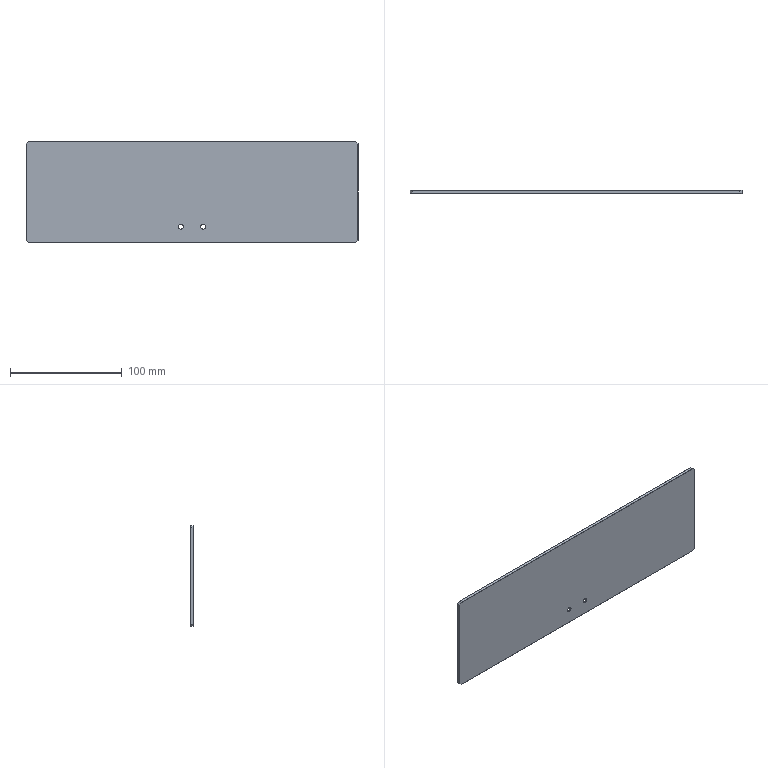Part | SolidWorks | features Chamfer 3, Extrusion 1, HoleWzd 1 | 1 solid | 34 faces | box 297 x 3 x 90 mm | volume 79946 mm3 | plane 26 | cone 4 | cylinder 4 | commonest cylinder face diameters 4.5 x4
STEP:
#1=CARTESIAN_POINT('',(-10.,0.77,-33.25));
#2=VERTEX_POINT('',#1);
#3=CARTESIAN_POINT('',(-10.,0.77,-28.75));
#4=VERTEX_POINT('',#3);
#5=CARTESIAN_POINT('',(-10.,0.77,-31.));
#6=DIRECTION('',(0.,1.,0.));
#7=DIRECTION('',(0.,0.,1.));
#8=AXIS2_PLACEMENT_3D('',#5,#6,#7);
#9=CIRCLE('',#8,2.25);
#10=EDGE_CURVE('',#2,#4,#9,.T.);
#11=ORIENTED_EDGE('',*,*,#10,.F.);
#12=CARTESIAN_POINT('',(-10.,3.,-35.48));
#13=VERTEX_POINT('',#12);
#14=CARTESIAN_POINT('',(-10.,3.,-35.48));
#15=DIRECTION('',(0.,0.7071,-0.7071));
#16=VECTOR('',#15,1000.);
#17=LINE('',#14,#16);
#18=EDGE_CURVE('',#2,#13,#17,.T.);
#19=ORIENTED_EDGE('',*,*,#18,.T.);
#20=CARTESIAN_POINT('',(-10.,3.,-26.52));
#21=VERTEX_POINT('',#20);
#22=CARTESIAN_POINT('',(-10.,3.,-31.));
#23=DIRECTION('',(0.,1.,0.));
#24=DIRECTION('',(0.,0.,1.));
#25=AXIS2_PLACEMENT_3D('',#22,#23,#24);
#26=CIRCLE('',#25,4.48);
#27=EDGE_CURVE('',#13,#21,#26,.T.);
#28=ORIENTED_EDGE('',*,*,#27,.T.);
#29=CARTESIAN_POINT('',(-10.,3.,-26.52));
#30=DIRECTION('',(0.,0.7071,0.7071));
#31=VECTOR('',#30,1000.);
#32=LINE('',#29,#31);
#33=EDGE_CURVE('',#4,#21,#32,.T.);
#34=ORIENTED_EDGE('',*,*,#33,.F.);
#35=EDGE_LOOP('',(#11,#19,#28,#34));
#36=FACE_OUTER_BOUND('',#35,.T.);
#37=CARTESIAN_POINT('',(-10.,3.,-31.));
#38=DIRECTION('',(0.,1.,0.));
#39=DIRECTION('',(0.,0.,1.));
#40=AXIS2_PLACEMENT_3D('',#37,#38,#39);
#41=CONICAL_SURFACE('',#40,4.48,0.7854);
#42=ADVANCED_FACE('',(#36),#41,.F.);
#43=CARTESIAN_POINT('',(-10.,0.,-33.25));
#44=VERTEX_POINT('',#43);
#45=CARTESIAN_POINT('',(-10.,0.,-28.75));
#46=VERTEX_POINT('',#45);
#47=CARTESIAN_POINT('',(-10.,0.,-31.));
#48=DIRECTION('',(0.,1.,0.));
#49=DIRECTION('',(0.,0.,1.));
#50=AXIS2_PLACEMENT_3D('',#47,#48,#49);
#51=CIRCLE('',#50,2.25);
#52=EDGE_CURVE('',#44,#46,#51,.T.);
#53=ORIENTED_EDGE('',*,*,#52,.F.);
#54=CARTESIAN_POINT('',(-10.,3.,-33.25));
#55=DIRECTION('',(0.,1.,0.));
#56=VECTOR('',#55,1000.);
#57=LINE('',#54,#56);
#58=EDGE_CURVE('',#44,#2,#57,.T.);
#59=ORIENTED_EDGE('',*,*,#58,.T.);
#60=ORIENTED_EDGE('',*,*,#10,.T.);
#61=CARTESIAN_POINT('',(-10.,3.,-28.75));
#62=DIRECTION('',(0.,1.,0.));
#63=VECTOR('',#62,1000.);
#64=LINE('',#61,#63);
#65=EDGE_CURVE('',#46,#4,#64,.T.);
#66=ORIENTED_EDGE('',*,*,#65,.F.);
#67=EDGE_LOOP('',(#53,#59,#60,#66));
#68=FACE_OUTER_BOUND('',#67,.T.);
#69=CARTESIAN_POINT('',(-10.,3.,-31.));
#70=DIRECTION('',(0.,1.,0.));
#71=DIRECTION('',(0.,0.,1.));
#72=AXIS2_PLACEMENT_3D('',#69,#70,#71);
#73=CYLINDRICAL_SURFACE('',#72,2.25);
#74=ADVANCED_FACE('',(#68),#73,.F.);
#75=CARTESIAN_POINT('',(10.,0.77,-33.25));
#76=VERTEX_POINT('',#75);
#77=CARTESIAN_POINT('',(10.,0.77,-28.75));
#78=VERTEX_POINT('',#77);
#79=CARTESIAN_POINT('',(10.,0.77,-31.));
#80=DIRECTION('',(0.,1.,0.));
#81=DIRECTION('',(0.,0.,1.));
#82=AXIS2_PLACEMENT_3D('',#79,#80,#81);
#83=CIRCLE('',#82,2.25);
#84=EDGE_CURVE('',#76,#78,#83,.T.);
#85=ORIENTED_EDGE('',*,*,#84,.F.);
#86=CARTESIAN_POINT('',(10.,3.,-35.48));
#87=VERTEX_POINT('',#86);
#88=CARTESIAN_POINT('',(10.,3.,-35.48));
#89=DIRECTION('',(0.,0.7071,-0.7071));
#90=VECTOR('',#89,1000.);
#91=LINE('',#88,#90);
#92=EDGE_CURVE('',#76,#87,#91,.T.);
#93=ORIENTED_EDGE('',*,*,#92,.T.);
#94=CARTESIAN_POINT('',(10.,3.,-26.52));
#95=VERTEX_POINT('',#94);
#96=CARTESIAN_POINT('',(10.,3.,-31.));
#97=DIRECTION('',(0.,1.,0.));
#98=DIRECTION('',(0.,0.,1.));
#99=AXIS2_PLACEMENT_3D('',#96,#97,#98);
#100=CIRCLE('',#99,4.48);
#101=EDGE_CURVE('',#87,#95,#100,.T.);
#102=ORIENTED_EDGE('',*,*,#101,.T.);
#103=CARTESIAN_POINT('',(10.,3.,-26.52));
#104=DIRECTION('',(0.,0.7071,0.7071));
#105=VECTOR('',#104,1000.);
#106=LINE('',#103,#105);
#107=EDGE_CURVE('',#78,#95,#106,.T.);
#108=ORIENTED_EDGE('',*,*,#107,.F.);
#109=EDGE_LOOP('',(#85,#93,#102,#108));
#110=FACE_OUTER_BOUND('',#109,.T.);
#111=CARTESIAN_POINT('',(10.,3.,-31.));
#112=DIRECTION('',(0.,1.,0.));
#113=DIRECTION('',(0.,0.,1.));
#114=AXIS2_PLACEMENT_3D('',#111,#112,#113);
#115=CONICAL_SURFACE('',#114,4.48,0.7854);
#116=ADVANCED_FACE('',(#110),#115,.F.);
#117=CARTESIAN_POINT('',(10.,0.,-33.25));
#118=VERTEX_POINT('',#117);
#119=CARTESIAN_POINT('',(10.,0.,-28.75));
#120=VERTEX_POINT('',#119);
#121=CARTESIAN_POINT('',(10.,0.,-31.));
#122=DIRECTION('',(0.,1.,0.));
#123=DIRECTION('',(0.,0.,1.));
#124=AXIS2_PLACEMENT_3D('',#121,#122,#123);
#125=CIRCLE('',#124,2.25);
#126=EDGE_CURVE('',#118,#120,#125,.T.);
#127=ORIENTED_EDGE('',*,*,#126,.F.);
#128=CARTESIAN_POINT('',(10.,3.,-33.25));
#129=DIRECTION('',(0.,1.,0.));
#130=VECTOR('',#129,1000.);
#131=LINE('',#128,#130);
#132=EDGE_CURVE('',#118,#76,#131,.T.);
#133=ORIENTED_EDGE('',*,*,#132,.T.);
#134=ORIENTED_EDGE('',*,*,#84,.T.);
#135=CARTESIAN_POINT('',(10.,3.,-28.75));
#136=DIRECTION('',(0.,1.,0.));
#137=VECTOR('',#136,1000.);
#138=LINE('',#135,#137);
#139=EDGE_CURVE('',#120,#78,#138,.T.);
#140=ORIENTED_EDGE('',*,*,#139,.F.);
#141=EDGE_LOOP('',(#127,#133,#134,#140));
#142=FACE_OUTER_BOUND('',#141,.T.);
#143=CARTESIAN_POINT('',(10.,3.,-31.));
#144=DIRECTION('',(0.,1.,0.));
#145=DIRECTION('',(0.,0.,1.));
#146=AXIS2_PLACEMENT_3D('',#143,#144,#145);
#147=CYLINDRICAL_SURFACE('',#146,2.25);
#148=ADVANCED_FACE('',(#142),#147,.F.);
#149=CARTESIAN_POINT('',(148.5,0.2,-43.));
#150=VERTEX_POINT('',#149);
#151=CARTESIAN_POINT('',(148.5,2.8,-43.));
#152=VERTEX_POINT('',#151);
#153=CARTESIAN_POINT('',(148.5,3.,-43.));
#154=DIRECTION('',(0.,1.,0.));
#155=VECTOR('',#154,1000.);
#156=LINE('',#153,#155);
#157=EDGE_CURVE('',#150,#152,#156,.T.);
#158=ORIENTED_EDGE('',*,*,#157,.T.);
#159=CARTESIAN_POINT('',(148.5,2.8,43.));
#160=VERTEX_POINT('',#159);
#161=CARTESIAN_POINT('',(148.5,2.8,43.));
#162=DIRECTION('',(0.,0.,1.));
#163=VECTOR('',#162,1000.);
#164=LINE('',#161,#163);
#165=EDGE_CURVE('',#152,#160,#164,.T.);
#166=ORIENTED_EDGE('',*,*,#165,.T.);
#167=CARTESIAN_POINT('',(148.5,0.2,43.));
#168=VERTEX_POINT('',#167);
#169=CARTESIAN_POINT('',(148.5,3.,43.));
#170=DIRECTION('',(0.,-1.,0.));
#171=VECTOR('',#170,1000.);
#172=LINE('',#169,#171);
#173=EDGE_CURVE('',#160,#168,#172,.T.);
#174=ORIENTED_EDGE('',*,*,#173,.T.);
#175=CARTESIAN_POINT('',(148.5,0.2,-45.));
#176=DIRECTION('',(0.,0.,-1.));
#177=VECTOR('',#176,1000.);
#178=LINE('',#175,#177);
#179=EDGE_CURVE('',#168,#150,#178,.T.);
#180=ORIENTED_EDGE('',*,*,#179,.T.);
#181=EDGE_LOOP('',(#158,#166,#174,#180));
#182=FACE_OUTER_BOUND('',#181,.T.);
#183=CARTESIAN_POINT('',(148.5,3.,-45.));
#184=DIRECTION('',(-1.,0.,0.));
#185=DIRECTION('',(0.,0.,1.));
#186=AXIS2_PLACEMENT_3D('',#183,#184,#185);
#187=PLANE('',#186);
#188=ADVANCED_FACE('',(#182),#187,.F.);
#189=CARTESIAN_POINT('',(-146.5,0.2,-45.));
#190=VERTEX_POINT('',#189);
#191=CARTESIAN_POINT('',(-146.5,2.8,-45.));
#192=VERTEX_POINT('',#191);
#193=CARTESIAN_POINT('',(-146.5,3.,-45.));
#194=DIRECTION('',(0.,1.,0.));
#195=VECTOR('',#194,1000.);
#196=LINE('',#193,#195);
#197=EDGE_CURVE('',#190,#192,#196,.T.);
#198=ORIENTED_EDGE('',*,*,#197,.T.);
#199=CARTESIAN_POINT('',(146.5,2.8,-45.));
#200=VERTEX_POINT('',#199);
#201=CARTESIAN_POINT('',(146.5,2.8,-45.));
#202=DIRECTION('',(1.,0.,0.));
#203=VECTOR('',#202,1000.);
#204=LINE('',#201,#203);
#205=EDGE_CURVE('',#192,#200,#204,.T.);
#206=ORIENTED_EDGE('',*,*,#205,.T.);
#207=CARTESIAN_POINT('',(146.5,0.2,-45.));
#208=VERTEX_POINT('',#207);
#209=CARTESIAN_POINT('',(146.5,3.,-45.));
#210=DIRECTION('',(0.,-1.,0.));
#211=VECTOR('',#210,1000.);
#212=LINE('',#209,#211);
#213=EDGE_CURVE('',#200,#208,#212,.T.);
#214=ORIENTED_EDGE('',*,*,#213,.T.);
#215=CARTESIAN_POINT('',(-148.5,0.2,-45.));
#216=DIRECTION('',(-1.,0.,0.));
#217=VECTOR('',#216,1000.);
#218=LINE('',#215,#217);
#219=EDGE_CURVE('',#208,#190,#218,.T.);
#220=ORIENTED_EDGE('',*,*,#219,.T.);
#221=EDGE_LOOP('',(#198,#206,#214,#220));
#222=FACE_OUTER_BOUND('',#221,.T.);
#223=CARTESIAN_POINT('',(-148.5,3.,-45.));
#224=DIRECTION('',(0.,0.,1.));
#225=DIRECTION('',(1.,0.,0.));
#226=AXIS2_PLACEMENT_3D('',#223,#224,#225);
#227=PLANE('',#226);
#228=ADVANCED_FACE('',(#222),#227,.F.);
#229=CARTESIAN_POINT('',(-148.5,0.2,43.));
#230=VERTEX_POINT('',#229);
#231=CARTESIAN_POINT('',(-148.5,2.8,43.));
#232=VERTEX_POINT('',#231);
#233=CARTESIAN_POINT('',(-148.5,3.,43.));
#234=DIRECTION('',(0.,1.,0.));
#235=VECTOR('',#234,1000.);
#236=LINE('',#233,#235);
#237=EDGE_CURVE('',#230,#232,#236,.T.);
#238=ORIENTED_EDGE('',*,*,#237,.T.);
#239=CARTESIAN_POINT('',(-148.5,2.8,-43.));
#240=VERTEX_POINT('',#239);
#241=CARTESIAN_POINT('',(-148.5,2.8,-43.));
#242=DIRECTION('',(0.,0.,-1.));
#243=VECTOR('',#242,1000.);
#244=LINE('',#241,#243);
#245=EDGE_CURVE('',#232,#240,#244,.T.);
#246=ORIENTED_EDGE('',*,*,#245,.T.);
#247=CARTESIAN_POINT('',(-148.5,0.2,-43.));
#248=VERTEX_POINT('',#247);
#249=CARTESIAN_POINT('',(-148.5,3.,-43.));
#250=DIRECTION('',(0.,-1.,0.));
#251=VECTOR('',#250,1000.);
#252=LINE('',#249,#251);
#253=EDGE_CURVE('',#240,#248,#252,.T.);
#254=ORIENTED_EDGE('',*,*,#253,.T.);
#255=CARTESIAN_POINT('',(-148.5,0.2,-45.));
#256=DIRECTION('',(0.,0.,1.));
#257=VECTOR('',#256,1000.);
#258=LINE('',#255,#257);
#259=EDGE_CURVE('',#248,#230,#258,.T.);
#260=ORIENTED_EDGE('',*,*,#259,.T.);
#261=EDGE_LOOP('',(#238,#246,#254,#260));
#262=FACE_OUTER_BOUND('',#261,.T.);
#263=CARTESIAN_POINT('',(-148.5,3.,-45.));
#264=DIRECTION('',(1.,0.,0.));
#265=DIRECTION('',(0.,0.,-1.));
#266=AXIS2_PLACEMENT_3D('',#263,#264,#265);
#267=PLANE('',#266);
#268=ADVANCED_FACE('',(#262),#267,.F.);
#269=CARTESIAN_POINT('',(146.5,0.2,45.));
#270=VERTEX_POINT('',#269);
#271=CARTESIAN_POINT('',(146.5,2.8,45.));
#272=VERTEX_POINT('',#271);
#273=CARTESIAN_POINT('',(146.5,3.,45.));
#274=DIRECTION('',(0.,1.,0.));
#275=VECTOR('',#274,1000.);
#276=LINE('',#273,#275);
#277=EDGE_CURVE('',#270,#272,#276,.T.);
#278=ORIENTED_EDGE('',*,*,#277,.T.);
#279=CARTESIAN_POINT('',(-146.5,2.8,45.));
#280=VERTEX_POINT('',#279);
#281=CARTESIAN_POINT('',(-146.5,2.8,45.));
#282=DIRECTION('',(-1.,0.,0.));
#283=VECTOR('',#282,1000.);
#284=LINE('',#281,#283);
#285=EDGE_CURVE('',#272,#280,#284,.T.);
#286=ORIENTED_EDGE('',*,*,#285,.T.);
#287=CARTESIAN_POINT('',(-146.5,0.2,45.));
#288=VERTEX_POINT('',#287);
#289=CARTESIAN_POINT('',(-146.5,3.,45.));
#290=DIRECTION('',(0.,-1.,0.));
#291=VECTOR('',#290,1000.);
#292=LINE('',#289,#291);
#293=EDGE_CURVE('',#280,#288,#292,.T.);
#294=ORIENTED_EDGE('',*,*,#293,.T.);
#295=CARTESIAN_POINT('',(-148.5,0.2,45.));
#296=DIRECTION('',(1.,0.,0.));
#297=VECTOR('',#296,1000.);
#298=LINE('',#295,#297);
#299=EDGE_CURVE('',#288,#270,#298,.T.);
#300=ORIENTED_EDGE('',*,*,#299,.T.);
#301=EDGE_LOOP('',(#278,#286,#294,#300));
#302=FACE_OUTER_BOUND('',#301,.T.);
#303=CARTESIAN_POINT('',(-148.5,3.,45.));
#304=DIRECTION('',(0.,0.,-1.));
#305=DIRECTION('',(-1.,0.,0.));
#306=AXIS2_PLACEMENT_3D('',#303,#304,#305);
#307=PLANE('',#306);
#308=ADVANCED_FACE('',(#302),#307,.F.);
#309=CARTESIAN_POINT('',(148.3,3.,42.917));
#310=VERTEX_POINT('',#309);
#311=CARTESIAN_POINT('',(148.3,3.,-42.917));
#312=VERTEX_POINT('',#311);
#313=CARTESIAN_POINT('',(148.3,3.,-43.));
#314=DIRECTION('',(0.,0.,-1.));
#315=VECTOR('',#314,1000.);
#316=LINE('',#313,#315);
#317=EDGE_CURVE('',#310,#312,#316,.T.);
#318=ORIENTED_EDGE('',*,*,#317,.T.);
#319=CARTESIAN_POINT('',(146.417,3.,-44.8));
#320=VERTEX_POINT('',#319);
#321=CARTESIAN_POINT('',(95.609,3.,-95.609));
#322=DIRECTION('',(-0.7071,0.,-0.7071));
#323=VECTOR('',#322,1000.);
#324=LINE('',#321,#323);
#325=EDGE_CURVE('',#312,#320,#324,.T.);
#326=ORIENTED_EDGE('',*,*,#325,.T.);
#327=CARTESIAN_POINT('',(-146.417,3.,-44.8));
#328=VERTEX_POINT('',#327);
#329=CARTESIAN_POINT('',(-146.5,3.,-44.8));
#330=DIRECTION('',(-1.,0.,0.));
#331=VECTOR('',#330,1000.);
#332=LINE('',#329,#331);
#333=EDGE_CURVE('',#320,#328,#332,.T.);
#334=ORIENTED_EDGE('',*,*,#333,.T.);
#335=CARTESIAN_POINT('',(-148.3,3.,-42.917));
#336=VERTEX_POINT('',#335);
#337=CARTESIAN_POINT('',(-95.609,3.,-95.609));
#338=DIRECTION('',(-0.7071,0.,0.7071));
#339=VECTOR('',#338,1000.);
#340=LINE('',#337,#339);
#341=EDGE_CURVE('',#328,#336,#340,.T.);
#342=ORIENTED_EDGE('',*,*,#341,.T.);
#343=CARTESIAN_POINT('',(-148.3,3.,42.917));
#344=VERTEX_POINT('',#343);
#345=CARTESIAN_POINT('',(-148.3,3.,43.));
#346=DIRECTION('',(0.,0.,1.));
#347=VECTOR('',#346,1000.);
#348=LINE('',#345,#347);
#349=EDGE_CURVE('',#336,#344,#348,.T.);
#350=ORIENTED_EDGE('',*,*,#349,.T.);
#351=CARTESIAN_POINT('',(-146.417,3.,44.8));
#352=VERTEX_POINT('',#351);
#353=CARTESIAN_POINT('',(-95.609,3.,95.609));
#354=DIRECTION('',(0.7071,0.,0.7071));
#355=VECTOR('',#354,1000.);
#356=LINE('',#353,#355);
#357=EDGE_CURVE('',#344,#352,#356,.T.);
#358=ORIENTED_EDGE('',*,*,#357,.T.);
#359=CARTESIAN_POINT('',(146.417,3.,44.8));
#360=VERTEX_POINT('',#359);
#361=CARTESIAN_POINT('',(146.5,3.,44.8));
#362=DIRECTION('',(1.,0.,0.));
#363=VECTOR('',#362,1000.);
#364=LINE('',#361,#363);
#365=EDGE_CURVE('',#352,#360,#364,.T.);
#366=ORIENTED_EDGE('',*,*,#365,.T.);
#367=CARTESIAN_POINT('',(95.609,3.,95.609));
#368=DIRECTION('',(0.7071,0.,-0.7071));
#369=VECTOR('',#368,1000.);
#370=LINE('',#367,#369);
#371=EDGE_CURVE('',#360,#310,#370,.T.);
#372=ORIENTED_EDGE('',*,*,#371,.T.);
#373=EDGE_LOOP('',(#318,#326,#334,#342,#350,#358,#366,#372));
#374=FACE_OUTER_BOUND('',#373,.T.);
#375=CARTESIAN_POINT('',(-10.,3.,-31.));
#376=DIRECTION('',(0.,1.,0.));
#377=DIRECTION('',(0.,0.,1.));
#378=AXIS2_PLACEMENT_3D('',#375,#376,#377);
#379=CIRCLE('',#378,4.48);
#380=EDGE_CURVE('',#21,#13,#379,.T.);
#381=ORIENTED_EDGE('',*,*,#380,.F.);
#382=ORIENTED_EDGE('',*,*,#27,.F.);
#383=EDGE_LOOP('',(#381,#382));
#384=FACE_BOUND('',#383,.T.);
#385=CARTESIAN_POINT('',(10.,3.,-31.));
#386=DIRECTION('',(0.,1.,0.));
#387=DIRECTION('',(0.,0.,1.));
#388=AXIS2_PLACEMENT_3D('',#385,#386,#387);
#389=CIRCLE('',#388,4.48);
#390=EDGE_CURVE('',#95,#87,#389,.T.);
#391=ORIENTED_EDGE('',*,*,#390,.F.);
#392=ORIENTED_EDGE('',*,*,#101,.F.);
#393=EDGE_LOOP('',(#391,#392));
#394=FACE_BOUND('',#393,.T.);
#395=CARTESIAN_POINT('',(0.,3.,0.));
#396=DIRECTION('',(0.,1.,0.));
#397=DIRECTION('',(0.,0.,1.));
#398=AXIS2_PLACEMENT_3D('',#395,#396,#397);
#399=PLANE('',#398);
#400=ADVANCED_FACE('',(#374,#384,#394),#399,.T.);
#401=CARTESIAN_POINT('',(146.417,0.,44.8));
#402=VERTEX_POINT('',#401);
#403=CARTESIAN_POINT('',(-146.417,0.,44.8));
#404=VERTEX_POINT('',#403);
#405=CARTESIAN_POINT('',(0.,0.,44.8));
#406=DIRECTION('',(-1.,0.,0.));
#407=VECTOR('',#406,1000.);
#408=LINE('',#405,#407);
#409=EDGE_CURVE('',#402,#404,#408,.T.);
#410=ORIENTED_EDGE('',*,*,#409,.T.);
#411=CARTESIAN_POINT('',(-148.3,0.,42.917));
#412=VERTEX_POINT('',#411);
#413=CARTESIAN_POINT('',(-148.359,0.,42.859));
#414=DIRECTION('',(-0.7071,0.,-0.7071));
#415=VECTOR('',#414,1000.);
#416=LINE('',#413,#415);
#417=EDGE_CURVE('',#404,#412,#416,.T.);
#418=ORIENTED_EDGE('',*,*,#417,.T.);
#419=CARTESIAN_POINT('',(-148.3,0.,-42.917));
#420=VERTEX_POINT('',#419);
#421=CARTESIAN_POINT('',(-148.3,0.,0.));
#422=DIRECTION('',(0.,0.,-1.));
#423=VECTOR('',#422,1000.);
#424=LINE('',#421,#423);
#425=EDGE_CURVE('',#412,#420,#424,.T.);
#426=ORIENTED_EDGE('',*,*,#425,.T.);
#427=CARTESIAN_POINT('',(-146.417,0.,-44.8));
#428=VERTEX_POINT('',#427);
#429=CARTESIAN_POINT('',(-146.359,0.,-44.859));
#430=DIRECTION('',(0.7071,0.,-0.7071));
#431=VECTOR('',#430,1000.);
#432=LINE('',#429,#431);
#433=EDGE_CURVE('',#420,#428,#432,.T.);
#434=ORIENTED_EDGE('',*,*,#433,.T.);
#435=CARTESIAN_POINT('',(146.417,0.,-44.8));
#436=VERTEX_POINT('',#435);
#437=CARTESIAN_POINT('',(0.,0.,-44.8));
#438=DIRECTION('',(1.,0.,0.));
#439=VECTOR('',#438,1000.);
#440=LINE('',#437,#439);
#441=EDGE_CURVE('',#428,#436,#440,.T.);
#442=ORIENTED_EDGE('',*,*,#441,.T.);
#443=CARTESIAN_POINT('',(148.3,0.,-42.917));
#444=VERTEX_POINT('',#443);
#445=CARTESIAN_POINT('',(148.359,0.,-42.859));
#446=DIRECTION('',(0.7071,0.,0.7071));
#447=VECTOR('',#446,1000.);
#448=LINE('',#445,#447);
#449=EDGE_CURVE('',#436,#444,#448,.T.);
#450=ORIENTED_EDGE('',*,*,#449,.T.);
#451=CARTESIAN_POINT('',(148.3,0.,42.917));
#452=VERTEX_POINT('',#451);
#453=CARTESIAN_POINT('',(148.3,0.,0.));
#454=DIRECTION('',(0.,0.,1.));
#455=VECTOR('',#454,1000.);
#456=LINE('',#453,#455);
#457=EDGE_CURVE('',#444,#452,#456,.T.);
#458=ORIENTED_EDGE('',*,*,#457,.T.);
#459=CARTESIAN_POINT('',(146.359,0.,44.859));
#460=DIRECTION('',(-0.7071,0.,0.7071));
#461=VECTOR('',#460,1000.);
#462=LINE('',#459,#461);
#463=EDGE_CURVE('',#452,#402,#462,.T.);
#464=ORIENTED_EDGE('',*,*,#463,.T.);
#465=EDGE_LOOP('',(#410,#418,#426,#434,#442,#450,#458,#464));
#466=FACE_OUTER_BOUND('',#465,.T.);
#467=CARTESIAN_POINT('',(-10.,0.,-31.));
#468=DIRECTION('',(0.,1.,0.));
#469=DIRECTION('',(0.,0.,1.));
#470=AXIS2_PLACEMENT_3D('',#467,#468,#469);
#471=CIRCLE('',#470,2.25);
#472=EDGE_CURVE('',#46,#44,#471,.T.);
#473=ORIENTED_EDGE('',*,*,#472,.T.);
#474=ORIENTED_EDGE('',*,*,#52,.T.);
#475=EDGE_LOOP('',(#473,#474));
#476=FACE_BOUND('',#475,.T.);
#477=CARTESIAN_POINT('',(10.,0.,-31.));
#478=DIRECTION('',(0.,1.,0.));
#479=DIRECTION('',(0.,0.,1.));
#480=AXIS2_PLACEMENT_3D('',#477,#478,#479);
#481=CIRCLE('',#480,2.25);
#482=EDGE_CURVE('',#120,#118,#481,.T.);
#483=ORIENTED_EDGE('',*,*,#482,.T.);
#484=ORIENTED_EDGE('',*,*,#126,.T.);
#485=EDGE_LOOP('',(#483,#484));
#486=FACE_BOUND('',#485,.T.);
#487=CARTESIAN_POINT('',(0.,0.,0.));
#488=DIRECTION('',(0.,1.,0.));
#489=DIRECTION('',(0.,0.,1.));
#490=AXIS2_PLACEMENT_3D('',#487,#488,#489);
#491=PLANE('',#490);
#492=ADVANCED_FACE('',(#466,#476,#486),#491,.F.);
#493=ORIENTED_EDGE('',*,*,#132,.F.);
#494=ORIENTED_EDGE('',*,*,#482,.F.);
#495=ORIENTED_EDGE('',*,*,#139,.T.);
#496=CARTESIAN_POINT('',(10.,0.77,-31.));
#497=DIRECTION('',(0.,1.,0.));
#498=DIRECTION('',(0.,0.,1.));
#499=AXIS2_PLACEMENT_3D('',#496,#497,#498);
#500=CIRCLE('',#499,2.25);
#501=EDGE_CURVE('',#78,#76,#500,.T.);
#502=ORIENTED_EDGE('',*,*,#501,.T.);
#503=EDGE_LOOP('',(#493,#494,#495,#502));
#504=FACE_OUTER_BOUND('',#503,.T.);
#505=CARTESIAN_POINT('',(10.,3.,-31.));
#506=DIRECTION('',(0.,1.,0.));
#507=DIRECTION('',(0.,0.,1.));
#508=AXIS2_PLACEMENT_3D('',#505,#506,#507);
#509=CYLINDRICAL_SURFACE('',#508,2.25);
#510=ADVANCED_FACE('',(#504),#509,.F.);
#511=ORIENTED_EDGE('',*,*,#92,.F.);
#512=ORIENTED_EDGE('',*,*,#501,.F.);
#513=ORIENTED_EDGE('',*,*,#107,.T.);
#514=ORIENTED_EDGE('',*,*,#390,.T.);
#515=EDGE_LOOP('',(#511,#512,#513,#514));
#516=FACE_OUTER_BOUND('',#515,.T.);
#517=CARTESIAN_POINT('',(10.,3.,-31.));
#518=DIRECTION('',(0.,1.,0.));
#519=DIRECTION('',(0.,0.,1.));
#520=AXIS2_PLACEMENT_3D('',#517,#518,#519);
#521=CONICAL_SURFACE('',#520,4.48,0.7854);
#522=ADVANCED_FACE('',(#516),#521,.F.);
#523=ORIENTED_EDGE('',*,*,#58,.F.);
#524=ORIENTED_EDGE('',*,*,#472,.F.);
#525=ORIENTED_EDGE('',*,*,#65,.T.);
#526=CARTESIAN_POINT('',(-10.,0.77,-31.));
#527=DIRECTION('',(0.,1.,0.));
#528=DIRECTION('',(0.,0.,1.));
#529=AXIS2_PLACEMENT_3D('',#526,#527,#528);
#530=CIRCLE('',#529,2.25);
#531=EDGE_CURVE('',#4,#2,#530,.T.);
#532=ORIENTED_EDGE('',*,*,#531,.T.);
#533=EDGE_LOOP('',(#523,#524,#525,#532));
#534=FACE_OUTER_BOUND('',#533,.T.);
#535=CARTESIAN_POINT('',(-10.,3.,-31.));
#536=DIRECTION('',(0.,1.,0.));
#537=DIRECTION('',(0.,0.,1.));
#538=AXIS2_PLACEMENT_3D('',#535,#536,#537);
#539=CYLINDRICAL_SURFACE('',#538,2.25);
#540=ADVANCED_FACE('',(#534),#539,.F.);
#541=ORIENTED_EDGE('',*,*,#18,.F.);
#542=ORIENTED_EDGE('',*,*,#531,.F.);
#543=ORIENTED_EDGE('',*,*,#33,.T.);
#544=ORIENTED_EDGE('',*,*,#380,.T.);
#545=EDGE_LOOP('',(#541,#542,#543,#544));
#546=FACE_OUTER_BOUND('',#545,.T.);
#547=CARTESIAN_POINT('',(-10.,3.,-31.));
#548=DIRECTION('',(0.,1.,0.));
#549=DIRECTION('',(0.,0.,1.));
#550=AXIS2_PLACEMENT_3D('',#547,#548,#549);
#551=CONICAL_SURFACE('',#550,4.48,0.7854);
#552=ADVANCED_FACE('',(#546),#551,.F.);
#553=ORIENTED_EDGE('',*,*,#213,.F.);
#554=CARTESIAN_POINT('',(146.5,2.8,-45.));
#555=DIRECTION('',(0.7071,0.,0.7071));
#556=VECTOR('',#555,1000.);
#557=LINE('',#554,#556);
#558=EDGE_CURVE('',#200,#152,#557,.T.);
#559=ORIENTED_EDGE('',*,*,#558,.T.);
#560=ORIENTED_EDGE('',*,*,#157,.F.);
#561=CARTESIAN_POINT('',(146.5,0.2,-45.));
#562=DIRECTION('',(-0.7071,0.,-0.7071));
#563=VECTOR('',#562,1000.);
#564=LINE('',#561,#563);
#565=EDGE_CURVE('',#150,#208,#564,.T.);
#566=ORIENTED_EDGE('',*,*,#565,.T.);
#567=EDGE_LOOP('',(#553,#559,#560,#566));
#568=FACE_OUTER_BOUND('',#567,.T.);
#569=CARTESIAN_POINT('',(146.5,3.,-45.));
#570=DIRECTION('',(-0.7071,0.,0.7071));
#571=DIRECTION('',(0.,-1.,0.));
#572=AXIS2_PLACEMENT_3D('',#569,#570,#571);
#573=PLANE('',#572);
#574=ADVANCED_FACE('',(#568),#573,.F.);
#575=ORIENTED_EDGE('',*,*,#173,.F.);
#576=CARTESIAN_POINT('',(148.5,2.8,43.));
#577=DIRECTION('',(-0.7071,0.,0.7071));
#578=VECTOR('',#577,1000.);
#579=LINE('',#576,#578);
#580=EDGE_CURVE('',#160,#272,#579,.T.);
#581=ORIENTED_EDGE('',*,*,#580,.T.);
#582=ORIENTED_EDGE('',*,*,#277,.F.);
#583=CARTESIAN_POINT('',(148.5,0.2,43.));
#584=DIRECTION('',(0.7071,0.,-0.7071));
#585=VECTOR('',#584,1000.);
#586=LINE('',#583,#585);
#587=EDGE_CURVE('',#270,#168,#586,.T.);
#588=ORIENTED_EDGE('',*,*,#587,.T.);
#589=EDGE_LOOP('',(#575,#581,#582,#588));
#590=FACE_OUTER_BOUND('',#589,.T.);
#591=CARTESIAN_POINT('',(148.5,3.,43.));
#592=DIRECTION('',(-0.7071,0.,-0.7071));
#593=DIRECTION('',(0.,-1.,0.));
#594=AXIS2_PLACEMENT_3D('',#591,#592,#593);
#595=PLANE('',#594);
#596=ADVANCED_FACE('',(#590),#595,.F.);
#597=ORIENTED_EDGE('',*,*,#293,.F.);
#598=CARTESIAN_POINT('',(-146.5,2.8,45.));
#599=DIRECTION('',(-0.7071,0.,-0.7071));
#600=VECTOR('',#599,1000.);
#601=LINE('',#598,#600);
#602=EDGE_CURVE('',#280,#232,#601,.T.);
#603=ORIENTED_EDGE('',*,*,#602,.T.);
#604=ORIENTED_EDGE('',*,*,#237,.F.);
#605=CARTESIAN_POINT('',(-146.5,0.2,45.));
#606=DIRECTION('',(0.7071,0.,0.7071));
#607=VECTOR('',#606,1000.);
#608=LINE('',#605,#607);
#609=EDGE_CURVE('',#230,#288,#608,.T.);
#610=ORIENTED_EDGE('',*,*,#609,.T.);
#611=EDGE_LOOP('',(#597,#603,#604,#610));
#612=FACE_OUTER_BOUND('',#611,.T.);
#613=CARTESIAN_POINT('',(-146.5,3.,45.));
#614=DIRECTION('',(0.7071,0.,-0.7071));
#615=DIRECTION('',(0.,-1.,0.));
#616=AXIS2_PLACEMENT_3D('',#613,#614,#615);
#617=PLANE('',#616);
#618=ADVANCED_FACE('',(#612),#617,.F.);
#619=ORIENTED_EDGE('',*,*,#253,.F.);
#620=CARTESIAN_POINT('',(-148.5,2.8,-43.));
#621=DIRECTION('',(0.7071,0.,-0.7071));
#622=VECTOR('',#621,1000.);
#623=LINE('',#620,#622);
#624=EDGE_CURVE('',#240,#192,#623,.T.);
#625=ORIENTED_EDGE('',*,*,#624,.T.);
#626=ORIENTED_EDGE('',*,*,#197,.F.);
#627=CARTESIAN_POINT('',(-148.5,0.2,-43.));
#628=DIRECTION('',(-0.7071,0.,0.7071));
#629=VECTOR('',#628,1000.);
#630=LINE('',#627,#629);
#631=EDGE_CURVE('',#190,#248,#630,.T.);
#632=ORIENTED_EDGE('',*,*,#631,.T.);
#633=EDGE_LOOP('',(#619,#625,#626,#632));
#634=FACE_OUTER_BOUND('',#633,.T.);
#635=CARTESIAN_POINT('',(-148.5,3.,-43.));
#636=DIRECTION('',(0.7071,0.,0.7071));
#637=DIRECTION('',(0.,-1.,0.));
#638=AXIS2_PLACEMENT_3D('',#635,#636,#637);
#639=PLANE('',#638);
#640=ADVANCED_FACE('',(#634),#639,.F.);
#641=CARTESIAN_POINT('',(123.192,-56.069,11.269));
#642=DIRECTION('',(-0.2811,-0.6786,0.6786));
#643=VECTOR('',#642,1000.);
#644=LINE('',#641,#643);
#645=EDGE_CURVE('',#208,#436,#644,.T.);
#646=ORIENTED_EDGE('',*,*,#645,.F.);
#647=ORIENTED_EDGE('',*,*,#565,.F.);
#648=CARTESIAN_POINT('',(134.086,-14.214,-37.03));
#649=DIRECTION('',(0.6786,0.6786,-0.2811));
#650=VECTOR('',#649,1000.);
#651=LINE('',#648,#650);
#652=EDGE_CURVE('',#444,#150,#651,.T.);
#653=ORIENTED_EDGE('',*,*,#652,.F.);
#654=ORIENTED_EDGE('',*,*,#449,.F.);
#655=EDGE_LOOP('',(#646,#647,#653,#654));
#656=FACE_OUTER_BOUND('',#655,.T.);
#657=CARTESIAN_POINT('',(95.609,0.,-95.609));
#658=DIRECTION('',(-0.5,0.7071,0.5));
#659=DIRECTION('',(0.7071,0.,0.7071));
#660=AXIS2_PLACEMENT_3D('',#657,#658,#659);
#661=PLANE('',#660);
#662=ADVANCED_FACE('',(#656),#661,.F.);
#663=ORIENTED_EDGE('',*,*,#652,.T.);
#664=ORIENTED_EDGE('',*,*,#179,.F.);
#665=CARTESIAN_POINT('',(131.715,-16.585,36.047));
#666=DIRECTION('',(0.6786,0.6786,0.2811));
#667=VECTOR('',#666,1000.);
#668=LINE('',#665,#667);
#669=EDGE_CURVE('',#452,#168,#668,.T.);
#670=ORIENTED_EDGE('',*,*,#669,.F.);
#671=ORIENTED_EDGE('',*,*,#457,.F.);
#672=EDGE_LOOP('',(#663,#664,#670,#671));
#673=FACE_OUTER_BOUND('',#672,.T.);
#674=CARTESIAN_POINT('',(148.5,0.2,-45.));
#675=DIRECTION('',(-0.7071,0.7071,0.));
#676=DIRECTION('',(0.,0.,-1.));
#677=AXIS2_PLACEMENT_3D('',#674,#675,#676);
#678=PLANE('',#677);
#679=ADVANCED_FACE('',(#673),#678,.F.);
#680=ORIENTED_EDGE('',*,*,#645,.T.);
#681=ORIENTED_EDGE('',*,*,#441,.F.);
#682=CARTESIAN_POINT('',(-152.094,13.706,-58.506));
#683=DIRECTION('',(0.2811,-0.6786,0.6786));
#684=VECTOR('',#683,1000.);
#685=LINE('',#682,#684);
#686=EDGE_CURVE('',#190,#428,#685,.T.);
#687=ORIENTED_EDGE('',*,*,#686,.F.);
#688=ORIENTED_EDGE('',*,*,#219,.F.);
#689=EDGE_LOOP('',(#680,#681,#687,#688));
#690=FACE_OUTER_BOUND('',#689,.T.);
#691=CARTESIAN_POINT('',(-148.5,0.2,-45.));
#692=DIRECTION('',(0.,0.7071,0.7071));
#693=DIRECTION('',(-1.,0.,0.));
#694=AXIS2_PLACEMENT_3D('',#691,#692,#693);
#695=PLANE('',#694);
#696=ADVANCED_FACE('',(#690),#695,.F.);
#697=ORIENTED_EDGE('',*,*,#669,.T.);
#698=ORIENTED_EDGE('',*,*,#587,.F.);
#699=CARTESIAN_POINT('',(152.094,13.706,58.506));
#700=DIRECTION('',(0.2811,0.6786,0.6786));
#701=VECTOR('',#700,1000.);
#702=LINE('',#699,#701);
#703=EDGE_CURVE('',#402,#270,#702,.T.);
#704=ORIENTED_EDGE('',*,*,#703,.F.);
#705=ORIENTED_EDGE('',*,*,#463,.F.);
#706=EDGE_LOOP('',(#697,#698,#704,#705));
#707=FACE_OUTER_BOUND('',#706,.T.);
#708=CARTESIAN_POINT('',(95.609,0.,95.609));
#709=DIRECTION('',(-0.5,0.7071,-0.5));
#710=DIRECTION('',(-0.7071,0.,0.7071));
#711=AXIS2_PLACEMENT_3D('',#708,#709,#710);
#712=PLANE('',#711);
#713=ADVANCED_FACE('',(#707),#712,.F.);
#714=ORIENTED_EDGE('',*,*,#686,.T.);
#715=ORIENTED_EDGE('',*,*,#433,.F.);
#716=CARTESIAN_POINT('',(-148.881,0.5815,-43.158));
#717=DIRECTION('',(0.6786,-0.6786,0.2811));
#718=VECTOR('',#717,1000.);
#719=LINE('',#716,#718);
#720=EDGE_CURVE('',#248,#420,#719,.T.);
#721=ORIENTED_EDGE('',*,*,#720,.F.);
#722=ORIENTED_EDGE('',*,*,#631,.F.);
#723=EDGE_LOOP('',(#714,#715,#721,#722));
#724=FACE_OUTER_BOUND('',#723,.T.);
#725=CARTESIAN_POINT('',(-95.609,0.,-95.609));
#726=DIRECTION('',(0.5,0.7071,0.5));
#727=DIRECTION('',(0.7071,0.,-0.7071));
#728=AXIS2_PLACEMENT_3D('',#725,#726,#727);
#729=PLANE('',#728);
#730=ADVANCED_FACE('',(#724),#729,.F.);
#731=ORIENTED_EDGE('',*,*,#703,.T.);
#732=ORIENTED_EDGE('',*,*,#299,.F.);
#733=CARTESIAN_POINT('',(-146.658,0.5815,45.381));
#734=DIRECTION('',(-0.2811,0.6786,0.6786));
#735=VECTOR('',#734,1000.);
#736=LINE('',#733,#735);
#737=EDGE_CURVE('',#404,#288,#736,.T.);
#738=ORIENTED_EDGE('',*,*,#737,.F.);
#739=ORIENTED_EDGE('',*,*,#409,.F.);
#740=EDGE_LOOP('',(#731,#732,#738,#739));
#741=FACE_OUTER_BOUND('',#740,.T.);
#742=CARTESIAN_POINT('',(-148.5,0.2,45.));
#743=DIRECTION('',(0.,0.7071,-0.7071));
#744=DIRECTION('',(1.,0.,0.));
#745=AXIS2_PLACEMENT_3D('',#742,#743,#744);
#746=PLANE('',#745);
#747=ADVANCED_FACE('',(#741),#746,.F.);
#748=ORIENTED_EDGE('',*,*,#720,.T.);
#749=ORIENTED_EDGE('',*,*,#425,.F.);
#750=CARTESIAN_POINT('',(-131.715,-16.585,36.047));
#751=DIRECTION('',(0.6786,-0.6786,-0.2811));
#752=VECTOR('',#751,1000.);
#753=LINE('',#750,#752);
#754=EDGE_CURVE('',#230,#412,#753,.T.);
#755=ORIENTED_EDGE('',*,*,#754,.F.);
#756=ORIENTED_EDGE('',*,*,#259,.F.);
#757=EDGE_LOOP('',(#748,#749,#755,#756));
#758=FACE_OUTER_BOUND('',#757,.T.);
#759=CARTESIAN_POINT('',(-148.5,0.2,-45.));
#760=DIRECTION('',(0.7071,0.7071,0.));
#761=DIRECTION('',(0.,0.,1.));
#762=AXIS2_PLACEMENT_3D('',#759,#760,#761);
#763=PLANE('',#762);
#764=ADVANCED_FACE('',(#758),#763,.F.);
#765=ORIENTED_EDGE('',*,*,#737,.T.);
#766=ORIENTED_EDGE('',*,*,#609,.F.);
#767=ORIENTED_EDGE('',*,*,#754,.T.);
#768=ORIENTED_EDGE('',*,*,#417,.F.);
#769=EDGE_LOOP('',(#765,#766,#767,#768));
#770=FACE_OUTER_BOUND('',#769,.T.);
#771=CARTESIAN_POINT('',(-95.609,0.,95.609));
#772=DIRECTION('',(0.5,0.7071,-0.5));
#773=DIRECTION('',(-0.7071,0.,-0.7071));
#774=AXIS2_PLACEMENT_3D('',#771,#772,#773);
#775=PLANE('',#774);
#776=ADVANCED_FACE('',(#770),#775,.F.);
#777=CARTESIAN_POINT('',(-140.114,11.186,39.526));
#778=DIRECTION('',(0.6786,0.6786,-0.2811));
#779=VECTOR('',#778,1000.);
#780=LINE('',#777,#779);
#781=EDGE_CURVE('',#232,#344,#780,.T.);
#782=ORIENTED_EDGE('',*,*,#781,.F.);
#783=ORIENTED_EDGE('',*,*,#602,.F.);
#784=CARTESIAN_POINT('',(-152.094,-10.706,58.506));
#785=DIRECTION('',(-0.2811,-0.6786,0.6786));
#786=VECTOR('',#785,1000.);
#787=LINE('',#784,#786);
#788=EDGE_CURVE('',#352,#280,#787,.T.);
#789=ORIENTED_EDGE('',*,*,#788,.F.);
#790=ORIENTED_EDGE('',*,*,#357,.F.);
#791=EDGE_LOOP('',(#782,#783,#789,#790));
#792=FACE_OUTER_BOUND('',#791,.T.);
#793=CARTESIAN_POINT('',(-95.609,3.,95.609));
#794=DIRECTION('',(-0.5,0.7071,0.5));
#795=DIRECTION('',(-0.7071,0.,-0.7071));
#796=AXIS2_PLACEMENT_3D('',#793,#794,#795);
#797=PLANE('',#796);
#798=ADVANCED_FACE('',(#792),#797,.T.);
#799=ORIENTED_EDGE('',*,*,#788,.T.);
#800=ORIENTED_EDGE('',*,*,#285,.F.);
#801=CARTESIAN_POINT('',(134.849,30.928,16.872));
#802=DIRECTION('',(0.2811,-0.6786,0.6786));
#803=VECTOR('',#802,1000.);
#804=LINE('',#801,#803);
#805=EDGE_CURVE('',#360,#272,#804,.T.);
#806=ORIENTED_EDGE('',*,*,#805,.F.);
#807=ORIENTED_EDGE('',*,*,#365,.F.);
#808=EDGE_LOOP('',(#799,#800,#806,#807));
#809=FACE_OUTER_BOUND('',#808,.T.);
#810=CARTESIAN_POINT('',(0.,3.,44.8));
#811=DIRECTION('',(0.,0.7071,0.7071));
#812=DIRECTION('',(-1.,0.,0.));
#813=AXIS2_PLACEMENT_3D('',#810,#811,#812);
#814=PLANE('',#813);
#815=ADVANCED_FACE('',(#809),#814,.T.);
#816=ORIENTED_EDGE('',*,*,#781,.T.);
#817=ORIENTED_EDGE('',*,*,#349,.F.);
#818=CARTESIAN_POINT('',(-134.086,17.214,-37.03));
#819=DIRECTION('',(0.6786,0.6786,0.2811));
#820=VECTOR('',#819,1000.);
#821=LINE('',#818,#820);
#822=EDGE_CURVE('',#240,#336,#821,.T.);
#823=ORIENTED_EDGE('',*,*,#822,.F.);
#824=ORIENTED_EDGE('',*,*,#245,.F.);
#825=EDGE_LOOP('',(#816,#817,#823,#824));
#826=FACE_OUTER_BOUND('',#825,.T.);
#827=CARTESIAN_POINT('',(-148.3,3.,0.));
#828=DIRECTION('',(-0.7071,0.7071,0.));
#829=DIRECTION('',(0.,0.,-1.));
#830=AXIS2_PLACEMENT_3D('',#827,#828,#829);
#831=PLANE('',#830);
#832=ADVANCED_FACE('',(#826),#831,.T.);
#833=ORIENTED_EDGE('',*,*,#805,.T.);
#834=ORIENTED_EDGE('',*,*,#580,.F.);
#835=CARTESIAN_POINT('',(134.086,17.214,37.03));
#836=DIRECTION('',(0.6786,-0.6786,0.2811));
#837=VECTOR('',#836,1000.);
#838=LINE('',#835,#837);
#839=EDGE_CURVE('',#310,#160,#838,.T.);
#840=ORIENTED_EDGE('',*,*,#839,.F.);
#841=ORIENTED_EDGE('',*,*,#371,.F.);
#842=EDGE_LOOP('',(#833,#834,#840,#841));
#843=FACE_OUTER_BOUND('',#842,.T.);
#844=CARTESIAN_POINT('',(95.609,3.,95.609));
#845=DIRECTION('',(0.5,0.7071,0.5));
#846=DIRECTION('',(-0.7071,0.,0.7071));
#847=AXIS2_PLACEMENT_3D('',#844,#845,#846);
#848=PLANE('',#847);
#849=ADVANCED_FACE('',(#843),#848,.T.);
#850=ORIENTED_EDGE('',*,*,#822,.T.);
#851=ORIENTED_EDGE('',*,*,#341,.F.);
#852=CARTESIAN_POINT('',(-134.849,30.928,-16.872));
#853=DIRECTION('',(0.2811,0.6786,0.6786));
#854=VECTOR('',#853,1000.);
#855=LINE('',#852,#854);
#856=EDGE_CURVE('',#192,#328,#855,.T.);
#857=ORIENTED_EDGE('',*,*,#856,.F.);
#858=ORIENTED_EDGE('',*,*,#624,.F.);
#859=EDGE_LOOP('',(#850,#851,#857,#858));
#860=FACE_OUTER_BOUND('',#859,.T.);
#861=CARTESIAN_POINT('',(-95.609,3.,-95.609));
#862=DIRECTION('',(-0.5,0.7071,-0.5));
#863=DIRECTION('',(0.7071,0.,-0.7071));
#864=AXIS2_PLACEMENT_3D('',#861,#862,#863);
#865=PLANE('',#864);
#866=ADVANCED_FACE('',(#860),#865,.T.);
#867=ORIENTED_EDGE('',*,*,#839,.T.);
#868=ORIENTED_EDGE('',*,*,#165,.F.);
#869=CARTESIAN_POINT('',(140.114,11.186,-39.526));
#870=DIRECTION('',(0.6786,-0.6786,-0.2811));
#871=VECTOR('',#870,1000.);
#872=LINE('',#869,#871);
#873=EDGE_CURVE('',#312,#152,#872,.T.);
#874=ORIENTED_EDGE('',*,*,#873,.F.);
#875=ORIENTED_EDGE('',*,*,#317,.F.);
#876=EDGE_LOOP('',(#867,#868,#874,#875));
#877=FACE_OUTER_BOUND('',#876,.T.);
#878=CARTESIAN_POINT('',(148.3,3.,0.));
#879=DIRECTION('',(0.7071,0.7071,0.));
#880=DIRECTION('',(0.,0.,1.));
#881=AXIS2_PLACEMENT_3D('',#878,#879,#880);
#882=PLANE('',#881);
#883=ADVANCED_FACE('',(#877),#882,.T.);
#884=ORIENTED_EDGE('',*,*,#856,.T.);
#885=ORIENTED_EDGE('',*,*,#333,.F.);
#886=CARTESIAN_POINT('',(134.849,30.928,-16.872));
#887=DIRECTION('',(-0.2811,0.6786,0.6786));
#888=VECTOR('',#887,1000.);
#889=LINE('',#886,#888);
#890=EDGE_CURVE('',#200,#320,#889,.T.);
#891=ORIENTED_EDGE('',*,*,#890,.F.);
#892=ORIENTED_EDGE('',*,*,#205,.F.);
#893=EDGE_LOOP('',(#884,#885,#891,#892));
#894=FACE_OUTER_BOUND('',#893,.T.);
#895=CARTESIAN_POINT('',(0.,3.,-44.8));
#896=DIRECTION('',(0.,0.7071,-0.7071));
#897=DIRECTION('',(1.,0.,0.));
#898=AXIS2_PLACEMENT_3D('',#895,#896,#897);
#899=PLANE('',#898);
#900=ADVANCED_FACE('',(#894),#899,.T.);
#901=ORIENTED_EDGE('',*,*,#873,.T.);
#902=ORIENTED_EDGE('',*,*,#558,.F.);
#903=ORIENTED_EDGE('',*,*,#890,.T.);
#904=ORIENTED_EDGE('',*,*,#325,.F.);
#905=EDGE_LOOP('',(#901,#902,#903,#904));
#906=FACE_OUTER_BOUND('',#905,.T.);
#907=CARTESIAN_POINT('',(95.609,3.,-95.609));
#908=DIRECTION('',(0.5,0.7071,-0.5));
#909=DIRECTION('',(0.7071,0.,0.7071));
#910=AXIS2_PLACEMENT_3D('',#907,#908,#909);
#911=PLANE('',#910);
#912=ADVANCED_FACE('',(#906),#911,.T.);
#913=CLOSED_SHELL('',(#42,#74,#116,#148,#188,#228,#268,#308,#400,#492,#510,#522,#540,#552,#574,#596,#618,#640,#662,#679,#696,#713,#730,#747,#764,#776,#798,#815,#832,#849,#866,#883,#900,#912));
#914=MANIFOLD_SOLID_BREP('',#913);
#915=CARTESIAN_POINT('',(0.,0.,0.));
#916=DIRECTION('',(0.,0.,1.));
#917=DIRECTION('',(1.,0.,0.));
#918=AXIS2_PLACEMENT_3D('',#915,#916,#917);
#919=(LENGTH_UNIT()NAMED_UNIT(*)SI_UNIT(.MILLI.,.METRE.));
#920=UNCERTAINTY_MEASURE_WITH_UNIT(LENGTH_MEASURE(0.00001),#919,'','');
#921=(NAMED_UNIT(*)PLANE_ANGLE_UNIT()SI_UNIT($,.RADIAN.));
#922=(NAMED_UNIT(*)SI_UNIT($,.STERADIAN.)SOLID_ANGLE_UNIT());
#923=(GEOMETRIC_REPRESENTATION_CONTEXT(3)GLOBAL_UNCERTAINTY_ASSIGNED_CONTEXT((#920))GLOBAL_UNIT_ASSIGNED_CONTEXT((#919,#921,#922))REPRESENTATION_CONTEXT('',''));
#924=ADVANCED_BREP_SHAPE_REPRESENTATION('',(#914,#918),#923);